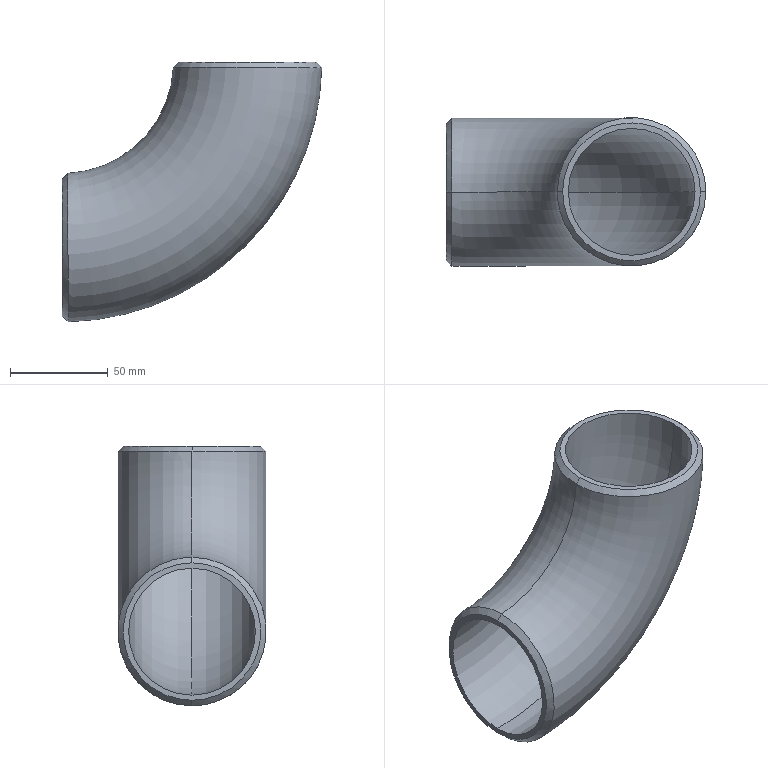Part | SolidWorks | features Chamfer 1, Revolution 1 | 1 solid | 10 faces | box 132.972 x 76 x 132.966 mm | volume 179855 mm3 | spline 4 | torus 4 | plane 2